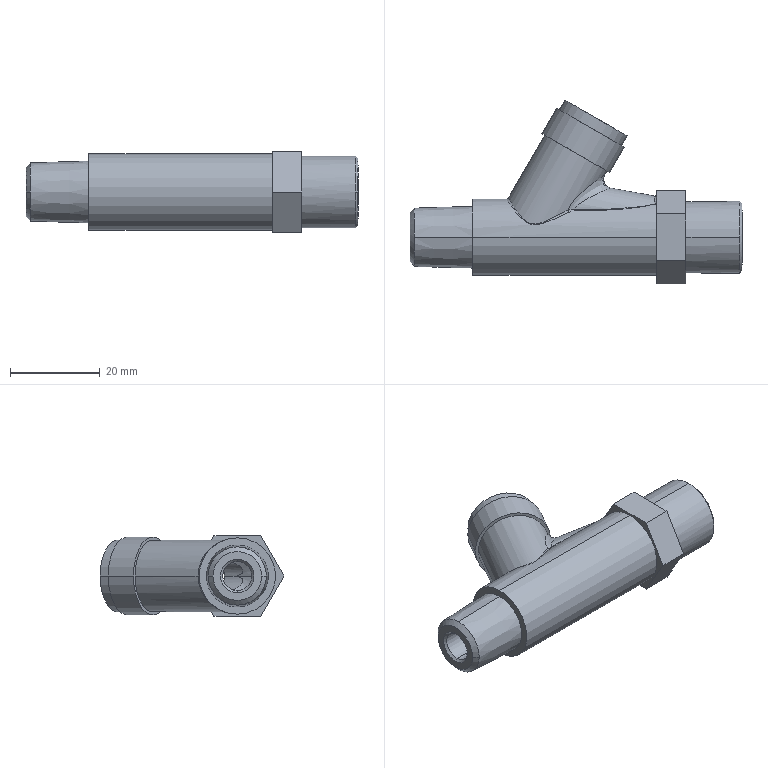Part | STEP file | 300221050#MCT225-08 | 1 solid | 70 faces | box 74 x 40.976 x 18 mm | volume 15654 mm3 | cylinder 26 | plane 17 | cone 16 | spline 11 | commonest cylinder face diameters 6.5 x10 16 x6 10.6 x2 12 x2 13.5 x2 17 x2